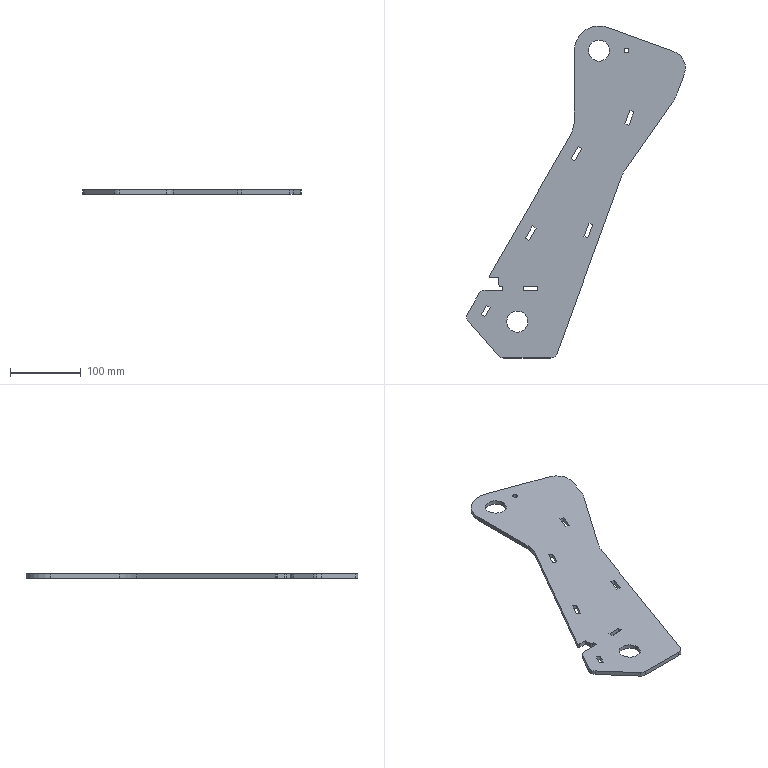Part | SolidWorks | features Fillet 3, FlatPattern 1, HoleWzd 1, SMBaseFlange 1, SheetMetal 1 | 1 solid | 59 faces | box 310.123 x 471.04 x 6 mm | volume 332793 mm3 | plane 40 | cylinder 19 | commonest cylinder face diameters 20 x5 30 x4 4 x3 100 x3 6.8 x2 50 x1